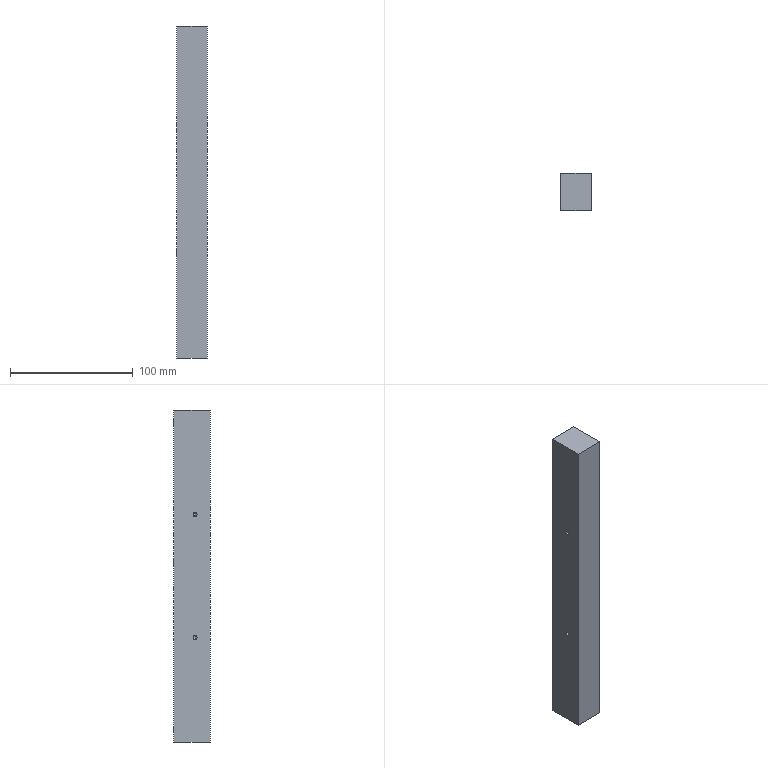Part | STEP file | 0243_209_Bar | 1 solid | 30 faces | box 25 x 30 x 270 mm | volume 201534 mm3 | cylinder 12 | cone 12 | plane 6 | commonest cylinder face diameters 3.3 x8 5 x4